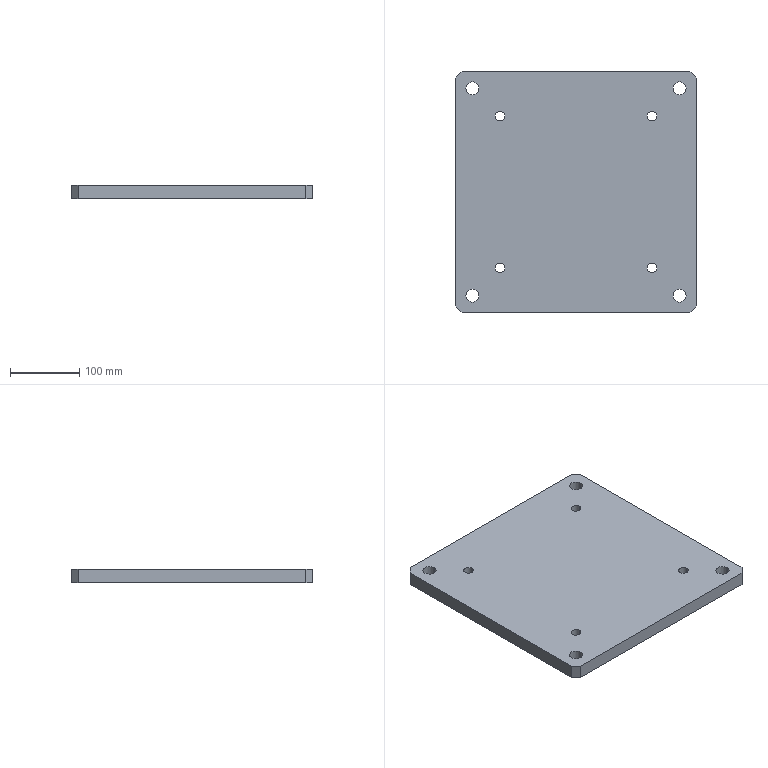Part | SolidWorks | features HoleWzd 2, Chamfer 1, Extrusion 1 | 1 solid | 26 faces | box 350 x 350 x 20 mm | volume 2411003 mm3 | cylinder 16 | plane 10 | commonest cylinder face diameters 14 x8 19 x8
STEP:
#1=CARTESIAN_POINT('',(140.5,150.,0.));
#2=VERTEX_POINT('',#1);
#3=CARTESIAN_POINT('',(159.5,150.,0.));
#4=VERTEX_POINT('',#3);
#5=CARTESIAN_POINT('',(150.,150.,0.));
#6=DIRECTION('',(0.,0.,1.));
#7=DIRECTION('',(1.,0.,0.));
#8=AXIS2_PLACEMENT_3D('',#5,#6,#7);
#9=CIRCLE('',#8,9.5);
#10=EDGE_CURVE('',#2,#4,#9,.T.);
#11=ORIENTED_EDGE('',*,*,#10,.F.);
#12=CARTESIAN_POINT('',(140.5,150.,20.));
#13=VERTEX_POINT('',#12);
#14=CARTESIAN_POINT('',(140.5,150.,20.));
#15=DIRECTION('',(0.,0.,1.));
#16=VECTOR('',#15,1000.);
#17=LINE('',#14,#16);
#18=EDGE_CURVE('',#2,#13,#17,.T.);
#19=ORIENTED_EDGE('',*,*,#18,.T.);
#20=CARTESIAN_POINT('',(159.5,150.,20.));
#21=VERTEX_POINT('',#20);
#22=CARTESIAN_POINT('',(150.,150.,20.));
#23=DIRECTION('',(0.,0.,1.));
#24=DIRECTION('',(1.,0.,0.));
#25=AXIS2_PLACEMENT_3D('',#22,#23,#24);
#26=CIRCLE('',#25,9.5);
#27=EDGE_CURVE('',#13,#21,#26,.T.);
#28=ORIENTED_EDGE('',*,*,#27,.T.);
#29=CARTESIAN_POINT('',(159.5,150.,20.));
#30=DIRECTION('',(0.,0.,1.));
#31=VECTOR('',#30,1000.);
#32=LINE('',#29,#31);
#33=EDGE_CURVE('',#4,#21,#32,.T.);
#34=ORIENTED_EDGE('',*,*,#33,.F.);
#35=EDGE_LOOP('',(#11,#19,#28,#34));
#36=FACE_OUTER_BOUND('',#35,.T.);
#37=CARTESIAN_POINT('',(150.,150.,20.));
#38=DIRECTION('',(0.,0.,1.));
#39=DIRECTION('',(1.,0.,0.));
#40=AXIS2_PLACEMENT_3D('',#37,#38,#39);
#41=CYLINDRICAL_SURFACE('',#40,9.5);
#42=ADVANCED_FACE('',(#36),#41,.F.);
#43=CARTESIAN_POINT('',(-159.5,-150.,0.));
#44=VERTEX_POINT('',#43);
#45=CARTESIAN_POINT('',(-140.5,-150.,0.));
#46=VERTEX_POINT('',#45);
#47=CARTESIAN_POINT('',(-150.,-150.,0.));
#48=DIRECTION('',(0.,0.,1.));
#49=DIRECTION('',(1.,0.,0.));
#50=AXIS2_PLACEMENT_3D('',#47,#48,#49);
#51=CIRCLE('',#50,9.5);
#52=EDGE_CURVE('',#44,#46,#51,.T.);
#53=ORIENTED_EDGE('',*,*,#52,.F.);
#54=CARTESIAN_POINT('',(-159.5,-150.,20.));
#55=VERTEX_POINT('',#54);
#56=CARTESIAN_POINT('',(-159.5,-150.,20.));
#57=DIRECTION('',(0.,0.,1.));
#58=VECTOR('',#57,1000.);
#59=LINE('',#56,#58);
#60=EDGE_CURVE('',#44,#55,#59,.T.);
#61=ORIENTED_EDGE('',*,*,#60,.T.);
#62=CARTESIAN_POINT('',(-140.5,-150.,20.));
#63=VERTEX_POINT('',#62);
#64=CARTESIAN_POINT('',(-150.,-150.,20.));
#65=DIRECTION('',(0.,0.,1.));
#66=DIRECTION('',(1.,0.,0.));
#67=AXIS2_PLACEMENT_3D('',#64,#65,#66);
#68=CIRCLE('',#67,9.5);
#69=EDGE_CURVE('',#55,#63,#68,.T.);
#70=ORIENTED_EDGE('',*,*,#69,.T.);
#71=CARTESIAN_POINT('',(-140.5,-150.,20.));
#72=DIRECTION('',(0.,0.,1.));
#73=VECTOR('',#72,1000.);
#74=LINE('',#71,#73);
#75=EDGE_CURVE('',#46,#63,#74,.T.);
#76=ORIENTED_EDGE('',*,*,#75,.F.);
#77=EDGE_LOOP('',(#53,#61,#70,#76));
#78=FACE_OUTER_BOUND('',#77,.T.);
#79=CARTESIAN_POINT('',(-150.,-150.,20.));
#80=DIRECTION('',(0.,0.,1.));
#81=DIRECTION('',(1.,0.,0.));
#82=AXIS2_PLACEMENT_3D('',#79,#80,#81);
#83=CYLINDRICAL_SURFACE('',#82,9.5);
#84=ADVANCED_FACE('',(#78),#83,.F.);
#85=CARTESIAN_POINT('',(-159.5,150.,0.));
#86=VERTEX_POINT('',#85);
#87=CARTESIAN_POINT('',(-140.5,150.,0.));
#88=VERTEX_POINT('',#87);
#89=CARTESIAN_POINT('',(-150.,150.,0.));
#90=DIRECTION('',(0.,0.,1.));
#91=DIRECTION('',(1.,0.,0.));
#92=AXIS2_PLACEMENT_3D('',#89,#90,#91);
#93=CIRCLE('',#92,9.5);
#94=EDGE_CURVE('',#86,#88,#93,.T.);
#95=ORIENTED_EDGE('',*,*,#94,.F.);
#96=CARTESIAN_POINT('',(-159.5,150.,20.));
#97=VERTEX_POINT('',#96);
#98=CARTESIAN_POINT('',(-159.5,150.,20.));
#99=DIRECTION('',(0.,0.,1.));
#100=VECTOR('',#99,1000.);
#101=LINE('',#98,#100);
#102=EDGE_CURVE('',#86,#97,#101,.T.);
#103=ORIENTED_EDGE('',*,*,#102,.T.);
#104=CARTESIAN_POINT('',(-140.5,150.,20.));
#105=VERTEX_POINT('',#104);
#106=CARTESIAN_POINT('',(-150.,150.,20.));
#107=DIRECTION('',(0.,0.,1.));
#108=DIRECTION('',(1.,0.,0.));
#109=AXIS2_PLACEMENT_3D('',#106,#107,#108);
#110=CIRCLE('',#109,9.5);
#111=EDGE_CURVE('',#97,#105,#110,.T.);
#112=ORIENTED_EDGE('',*,*,#111,.T.);
#113=CARTESIAN_POINT('',(-140.5,150.,20.));
#114=DIRECTION('',(0.,0.,1.));
#115=VECTOR('',#114,1000.);
#116=LINE('',#113,#115);
#117=EDGE_CURVE('',#88,#105,#116,.T.);
#118=ORIENTED_EDGE('',*,*,#117,.F.);
#119=EDGE_LOOP('',(#95,#103,#112,#118));
#120=FACE_OUTER_BOUND('',#119,.T.);
#121=CARTESIAN_POINT('',(-150.,150.,20.));
#122=DIRECTION('',(0.,0.,1.));
#123=DIRECTION('',(1.,0.,0.));
#124=AXIS2_PLACEMENT_3D('',#121,#122,#123);
#125=CYLINDRICAL_SURFACE('',#124,9.5);
#126=ADVANCED_FACE('',(#120),#125,.F.);
#127=CARTESIAN_POINT('',(140.5,-150.,0.));
#128=VERTEX_POINT('',#127);
#129=CARTESIAN_POINT('',(159.5,-150.,0.));
#130=VERTEX_POINT('',#129);
#131=CARTESIAN_POINT('',(150.,-150.,0.));
#132=DIRECTION('',(0.,0.,1.));
#133=DIRECTION('',(1.,0.,0.));
#134=AXIS2_PLACEMENT_3D('',#131,#132,#133);
#135=CIRCLE('',#134,9.5);
#136=EDGE_CURVE('',#128,#130,#135,.T.);
#137=ORIENTED_EDGE('',*,*,#136,.F.);
#138=CARTESIAN_POINT('',(140.5,-150.,20.));
#139=VERTEX_POINT('',#138);
#140=CARTESIAN_POINT('',(140.5,-150.,20.));
#141=DIRECTION('',(0.,0.,1.));
#142=VECTOR('',#141,1000.);
#143=LINE('',#140,#142);
#144=EDGE_CURVE('',#128,#139,#143,.T.);
#145=ORIENTED_EDGE('',*,*,#144,.T.);
#146=CARTESIAN_POINT('',(159.5,-150.,20.));
#147=VERTEX_POINT('',#146);
#148=CARTESIAN_POINT('',(150.,-150.,20.));
#149=DIRECTION('',(0.,0.,1.));
#150=DIRECTION('',(1.,0.,0.));
#151=AXIS2_PLACEMENT_3D('',#148,#149,#150);
#152=CIRCLE('',#151,9.5);
#153=EDGE_CURVE('',#139,#147,#152,.T.);
#154=ORIENTED_EDGE('',*,*,#153,.T.);
#155=CARTESIAN_POINT('',(159.5,-150.,20.));
#156=DIRECTION('',(0.,0.,1.));
#157=VECTOR('',#156,1000.);
#158=LINE('',#155,#157);
#159=EDGE_CURVE('',#130,#147,#158,.T.);
#160=ORIENTED_EDGE('',*,*,#159,.F.);
#161=EDGE_LOOP('',(#137,#145,#154,#160));
#162=FACE_OUTER_BOUND('',#161,.T.);
#163=CARTESIAN_POINT('',(150.,-150.,20.));
#164=DIRECTION('',(0.,0.,1.));
#165=DIRECTION('',(1.,0.,0.));
#166=AXIS2_PLACEMENT_3D('',#163,#164,#165);
#167=CYLINDRICAL_SURFACE('',#166,9.5);
#168=ADVANCED_FACE('',(#162),#167,.F.);
#169=CARTESIAN_POINT('',(103.,110.,0.));
#170=VERTEX_POINT('',#169);
#171=CARTESIAN_POINT('',(117.,110.,0.));
#172=VERTEX_POINT('',#171);
#173=CARTESIAN_POINT('',(110.,110.,0.));
#174=DIRECTION('',(0.,0.,1.));
#175=DIRECTION('',(1.,0.,0.));
#176=AXIS2_PLACEMENT_3D('',#173,#174,#175);
#177=CIRCLE('',#176,7.);
#178=EDGE_CURVE('',#170,#172,#177,.T.);
#179=ORIENTED_EDGE('',*,*,#178,.F.);
#180=CARTESIAN_POINT('',(103.,110.,20.));
#181=VERTEX_POINT('',#180);
#182=CARTESIAN_POINT('',(103.,110.,20.));
#183=DIRECTION('',(0.,0.,1.));
#184=VECTOR('',#183,1000.);
#185=LINE('',#182,#184);
#186=EDGE_CURVE('',#170,#181,#185,.T.);
#187=ORIENTED_EDGE('',*,*,#186,.T.);
#188=CARTESIAN_POINT('',(117.,110.,20.));
#189=VERTEX_POINT('',#188);
#190=CARTESIAN_POINT('',(110.,110.,20.));
#191=DIRECTION('',(0.,0.,1.));
#192=DIRECTION('',(1.,0.,0.));
#193=AXIS2_PLACEMENT_3D('',#190,#191,#192);
#194=CIRCLE('',#193,7.);
#195=EDGE_CURVE('',#181,#189,#194,.T.);
#196=ORIENTED_EDGE('',*,*,#195,.T.);
#197=CARTESIAN_POINT('',(117.,110.,20.));
#198=DIRECTION('',(0.,0.,1.));
#199=VECTOR('',#198,1000.);
#200=LINE('',#197,#199);
#201=EDGE_CURVE('',#172,#189,#200,.T.);
#202=ORIENTED_EDGE('',*,*,#201,.F.);
#203=EDGE_LOOP('',(#179,#187,#196,#202));
#204=FACE_OUTER_BOUND('',#203,.T.);
#205=CARTESIAN_POINT('',(110.,110.,20.));
#206=DIRECTION('',(0.,0.,1.));
#207=DIRECTION('',(1.,0.,0.));
#208=AXIS2_PLACEMENT_3D('',#205,#206,#207);
#209=CYLINDRICAL_SURFACE('',#208,7.);
#210=ADVANCED_FACE('',(#204),#209,.F.);
#211=CARTESIAN_POINT('',(-117.,-110.,0.));
#212=VERTEX_POINT('',#211);
#213=CARTESIAN_POINT('',(-103.,-110.,0.));
#214=VERTEX_POINT('',#213);
#215=CARTESIAN_POINT('',(-110.,-110.,0.));
#216=DIRECTION('',(0.,0.,1.));
#217=DIRECTION('',(1.,0.,0.));
#218=AXIS2_PLACEMENT_3D('',#215,#216,#217);
#219=CIRCLE('',#218,7.);
#220=EDGE_CURVE('',#212,#214,#219,.T.);
#221=ORIENTED_EDGE('',*,*,#220,.F.);
#222=CARTESIAN_POINT('',(-117.,-110.,20.));
#223=VERTEX_POINT('',#222);
#224=CARTESIAN_POINT('',(-117.,-110.,20.));
#225=DIRECTION('',(0.,0.,1.));
#226=VECTOR('',#225,1000.);
#227=LINE('',#224,#226);
#228=EDGE_CURVE('',#212,#223,#227,.T.);
#229=ORIENTED_EDGE('',*,*,#228,.T.);
#230=CARTESIAN_POINT('',(-103.,-110.,20.));
#231=VERTEX_POINT('',#230);
#232=CARTESIAN_POINT('',(-110.,-110.,20.));
#233=DIRECTION('',(0.,0.,1.));
#234=DIRECTION('',(1.,0.,0.));
#235=AXIS2_PLACEMENT_3D('',#232,#233,#234);
#236=CIRCLE('',#235,7.);
#237=EDGE_CURVE('',#223,#231,#236,.T.);
#238=ORIENTED_EDGE('',*,*,#237,.T.);
#239=CARTESIAN_POINT('',(-103.,-110.,20.));
#240=DIRECTION('',(0.,0.,1.));
#241=VECTOR('',#240,1000.);
#242=LINE('',#239,#241);
#243=EDGE_CURVE('',#214,#231,#242,.T.);
#244=ORIENTED_EDGE('',*,*,#243,.F.);
#245=EDGE_LOOP('',(#221,#229,#238,#244));
#246=FACE_OUTER_BOUND('',#245,.T.);
#247=CARTESIAN_POINT('',(-110.,-110.,20.));
#248=DIRECTION('',(0.,0.,1.));
#249=DIRECTION('',(1.,0.,0.));
#250=AXIS2_PLACEMENT_3D('',#247,#248,#249);
#251=CYLINDRICAL_SURFACE('',#250,7.);
#252=ADVANCED_FACE('',(#246),#251,.F.);
#253=CARTESIAN_POINT('',(-117.,110.,0.));
#254=VERTEX_POINT('',#253);
#255=CARTESIAN_POINT('',(-103.,110.,0.));
#256=VERTEX_POINT('',#255);
#257=CARTESIAN_POINT('',(-110.,110.,0.));
#258=DIRECTION('',(0.,0.,1.));
#259=DIRECTION('',(1.,0.,0.));
#260=AXIS2_PLACEMENT_3D('',#257,#258,#259);
#261=CIRCLE('',#260,7.);
#262=EDGE_CURVE('',#254,#256,#261,.T.);
#263=ORIENTED_EDGE('',*,*,#262,.F.);
#264=CARTESIAN_POINT('',(-117.,110.,20.));
#265=VERTEX_POINT('',#264);
#266=CARTESIAN_POINT('',(-117.,110.,20.));
#267=DIRECTION('',(0.,0.,1.));
#268=VECTOR('',#267,1000.);
#269=LINE('',#266,#268);
#270=EDGE_CURVE('',#254,#265,#269,.T.);
#271=ORIENTED_EDGE('',*,*,#270,.T.);
#272=CARTESIAN_POINT('',(-103.,110.,20.));
#273=VERTEX_POINT('',#272);
#274=CARTESIAN_POINT('',(-110.,110.,20.));
#275=DIRECTION('',(0.,0.,1.));
#276=DIRECTION('',(1.,0.,0.));
#277=AXIS2_PLACEMENT_3D('',#274,#275,#276);
#278=CIRCLE('',#277,7.);
#279=EDGE_CURVE('',#265,#273,#278,.T.);
#280=ORIENTED_EDGE('',*,*,#279,.T.);
#281=CARTESIAN_POINT('',(-103.,110.,20.));
#282=DIRECTION('',(0.,0.,1.));
#283=VECTOR('',#282,1000.);
#284=LINE('',#281,#283);
#285=EDGE_CURVE('',#256,#273,#284,.T.);
#286=ORIENTED_EDGE('',*,*,#285,.F.);
#287=EDGE_LOOP('',(#263,#271,#280,#286));
#288=FACE_OUTER_BOUND('',#287,.T.);
#289=CARTESIAN_POINT('',(-110.,110.,20.));
#290=DIRECTION('',(0.,0.,1.));
#291=DIRECTION('',(1.,0.,0.));
#292=AXIS2_PLACEMENT_3D('',#289,#290,#291);
#293=CYLINDRICAL_SURFACE('',#292,7.);
#294=ADVANCED_FACE('',(#288),#293,.F.);
#295=CARTESIAN_POINT('',(103.,-110.,0.));
#296=VERTEX_POINT('',#295);
#297=CARTESIAN_POINT('',(117.,-110.,0.));
#298=VERTEX_POINT('',#297);
#299=CARTESIAN_POINT('',(110.,-110.,0.));
#300=DIRECTION('',(0.,0.,1.));
#301=DIRECTION('',(1.,0.,0.));
#302=AXIS2_PLACEMENT_3D('',#299,#300,#301);
#303=CIRCLE('',#302,7.);
#304=EDGE_CURVE('',#296,#298,#303,.T.);
#305=ORIENTED_EDGE('',*,*,#304,.F.);
#306=CARTESIAN_POINT('',(103.,-110.,20.));
#307=VERTEX_POINT('',#306);
#308=CARTESIAN_POINT('',(103.,-110.,20.));
#309=DIRECTION('',(0.,0.,1.));
#310=VECTOR('',#309,1000.);
#311=LINE('',#308,#310);
#312=EDGE_CURVE('',#296,#307,#311,.T.);
#313=ORIENTED_EDGE('',*,*,#312,.T.);
#314=CARTESIAN_POINT('',(117.,-110.,20.));
#315=VERTEX_POINT('',#314);
#316=CARTESIAN_POINT('',(110.,-110.,20.));
#317=DIRECTION('',(0.,0.,1.));
#318=DIRECTION('',(1.,0.,0.));
#319=AXIS2_PLACEMENT_3D('',#316,#317,#318);
#320=CIRCLE('',#319,7.);
#321=EDGE_CURVE('',#307,#315,#320,.T.);
#322=ORIENTED_EDGE('',*,*,#321,.T.);
#323=CARTESIAN_POINT('',(117.,-110.,20.));
#324=DIRECTION('',(0.,0.,1.));
#325=VECTOR('',#324,1000.);
#326=LINE('',#323,#325);
#327=EDGE_CURVE('',#298,#315,#326,.T.);
#328=ORIENTED_EDGE('',*,*,#327,.F.);
#329=EDGE_LOOP('',(#305,#313,#322,#328));
#330=FACE_OUTER_BOUND('',#329,.T.);
#331=CARTESIAN_POINT('',(110.,-110.,20.));
#332=DIRECTION('',(0.,0.,1.));
#333=DIRECTION('',(1.,0.,0.));
#334=AXIS2_PLACEMENT_3D('',#331,#332,#333);
#335=CYLINDRICAL_SURFACE('',#334,7.);
#336=ADVANCED_FACE('',(#330),#335,.F.);
#337=CARTESIAN_POINT('',(175.,-165.,20.));
#338=VERTEX_POINT('',#337);
#339=CARTESIAN_POINT('',(175.,165.,20.));
#340=VERTEX_POINT('',#339);
#341=CARTESIAN_POINT('',(175.,175.,20.));
#342=DIRECTION('',(0.,1.,0.));
#343=VECTOR('',#342,1000.);
#344=LINE('',#341,#343);
#345=EDGE_CURVE('',#338,#340,#344,.T.);
#346=ORIENTED_EDGE('',*,*,#345,.F.);
#347=CARTESIAN_POINT('',(175.,-165.,0.));
#348=VERTEX_POINT('',#347);
#349=CARTESIAN_POINT('',(175.,-165.,20.));
#350=DIRECTION('',(0.,0.,-1.));
#351=VECTOR('',#350,1000.);
#352=LINE('',#349,#351);
#353=EDGE_CURVE('',#338,#348,#352,.T.);
#354=ORIENTED_EDGE('',*,*,#353,.T.);
#355=CARTESIAN_POINT('',(175.,165.,0.));
#356=VERTEX_POINT('',#355);
#357=CARTESIAN_POINT('',(175.,175.,0.));
#358=DIRECTION('',(0.,1.,0.));
#359=VECTOR('',#358,1000.);
#360=LINE('',#357,#359);
#361=EDGE_CURVE('',#348,#356,#360,.T.);
#362=ORIENTED_EDGE('',*,*,#361,.T.);
#363=CARTESIAN_POINT('',(175.,165.,20.));
#364=DIRECTION('',(0.,0.,1.));
#365=VECTOR('',#364,1000.);
#366=LINE('',#363,#365);
#367=EDGE_CURVE('',#356,#340,#366,.T.);
#368=ORIENTED_EDGE('',*,*,#367,.T.);
#369=EDGE_LOOP('',(#346,#354,#362,#368));
#370=FACE_OUTER_BOUND('',#369,.T.);
#371=CARTESIAN_POINT('',(175.,175.,20.));
#372=DIRECTION('',(-1.,0.,0.));
#373=DIRECTION('',(0.,0.,1.));
#374=AXIS2_PLACEMENT_3D('',#371,#372,#373);
#375=PLANE('',#374);
#376=ADVANCED_FACE('',(#370),#375,.F.);
#377=CARTESIAN_POINT('',(165.,175.,20.));
#378=VERTEX_POINT('',#377);
#379=CARTESIAN_POINT('',(-165.,175.,20.));
#380=VERTEX_POINT('',#379);
#381=CARTESIAN_POINT('',(-175.,175.,20.));
#382=DIRECTION('',(-1.,0.,0.));
#383=VECTOR('',#382,1000.);
#384=LINE('',#381,#383);
#385=EDGE_CURVE('',#378,#380,#384,.T.);
#386=ORIENTED_EDGE('',*,*,#385,.F.);
#387=CARTESIAN_POINT('',(165.,175.,0.));
#388=VERTEX_POINT('',#387);
#389=CARTESIAN_POINT('',(165.,175.,20.));
#390=DIRECTION('',(0.,0.,-1.));
#391=VECTOR('',#390,1000.);
#392=LINE('',#389,#391);
#393=EDGE_CURVE('',#378,#388,#392,.T.);
#394=ORIENTED_EDGE('',*,*,#393,.T.);
#395=CARTESIAN_POINT('',(-165.,175.,0.));
#396=VERTEX_POINT('',#395);
#397=CARTESIAN_POINT('',(-175.,175.,0.));
#398=DIRECTION('',(-1.,0.,0.));
#399=VECTOR('',#398,1000.);
#400=LINE('',#397,#399);
#401=EDGE_CURVE('',#388,#396,#400,.T.);
#402=ORIENTED_EDGE('',*,*,#401,.T.);
#403=CARTESIAN_POINT('',(-165.,175.,20.));
#404=DIRECTION('',(0.,0.,1.));
#405=VECTOR('',#404,1000.);
#406=LINE('',#403,#405);
#407=EDGE_CURVE('',#396,#380,#406,.T.);
#408=ORIENTED_EDGE('',*,*,#407,.T.);
#409=EDGE_LOOP('',(#386,#394,#402,#408));
#410=FACE_OUTER_BOUND('',#409,.T.);
#411=CARTESIAN_POINT('',(-175.,175.,20.));
#412=DIRECTION('',(0.,-1.,0.));
#413=DIRECTION('',(0.,0.,-1.));
#414=AXIS2_PLACEMENT_3D('',#411,#412,#413);
#415=PLANE('',#414);
#416=ADVANCED_FACE('',(#410),#415,.F.);
#417=CARTESIAN_POINT('',(-175.,165.,0.));
#418=VERTEX_POINT('',#417);
#419=CARTESIAN_POINT('',(-175.,-165.,0.));
#420=VERTEX_POINT('',#419);
#421=CARTESIAN_POINT('',(-175.,175.,0.));
#422=DIRECTION('',(0.,-1.,0.));
#423=VECTOR('',#422,1000.);
#424=LINE('',#421,#423);
#425=EDGE_CURVE('',#418,#420,#424,.T.);
#426=ORIENTED_EDGE('',*,*,#425,.T.);
#427=CARTESIAN_POINT('',(-175.,-165.,20.));
#428=VERTEX_POINT('',#427);
#429=CARTESIAN_POINT('',(-175.,-165.,20.));
#430=DIRECTION('',(0.,0.,1.));
#431=VECTOR('',#430,1000.);
#432=LINE('',#429,#431);
#433=EDGE_CURVE('',#420,#428,#432,.T.);
#434=ORIENTED_EDGE('',*,*,#433,.T.);
#435=CARTESIAN_POINT('',(-175.,165.,20.));
#436=VERTEX_POINT('',#435);
#437=CARTESIAN_POINT('',(-175.,175.,20.));
#438=DIRECTION('',(0.,-1.,0.));
#439=VECTOR('',#438,1000.);
#440=LINE('',#437,#439);
#441=EDGE_CURVE('',#436,#428,#440,.T.);
#442=ORIENTED_EDGE('',*,*,#441,.F.);
#443=CARTESIAN_POINT('',(-175.,165.,20.));
#444=DIRECTION('',(0.,0.,-1.));
#445=VECTOR('',#444,1000.);
#446=LINE('',#443,#445);
#447=EDGE_CURVE('',#436,#418,#446,.T.);
#448=ORIENTED_EDGE('',*,*,#447,.T.);
#449=EDGE_LOOP('',(#426,#434,#442,#448));
#450=FACE_OUTER_BOUND('',#449,.T.);
#451=CARTESIAN_POINT('',(-175.,175.,20.));
#452=DIRECTION('',(1.,0.,0.));
#453=DIRECTION('',(0.,0.,-1.));
#454=AXIS2_PLACEMENT_3D('',#451,#452,#453);
#455=PLANE('',#454);
#456=ADVANCED_FACE('',(#450),#455,.F.);
#457=CARTESIAN_POINT('',(-165.,-175.,20.));
#458=VERTEX_POINT('',#457);
#459=CARTESIAN_POINT('',(165.,-175.,20.));
#460=VERTEX_POINT('',#459);
#461=CARTESIAN_POINT('',(-175.,-175.,20.));
#462=DIRECTION('',(1.,0.,0.));
#463=VECTOR('',#462,1000.);
#464=LINE('',#461,#463);
#465=EDGE_CURVE('',#458,#460,#464,.T.);
#466=ORIENTED_EDGE('',*,*,#465,.F.);
#467=CARTESIAN_POINT('',(-165.,-175.,0.));
#468=VERTEX_POINT('',#467);
#469=CARTESIAN_POINT('',(-165.,-175.,20.));
#470=DIRECTION('',(0.,0.,-1.));
#471=VECTOR('',#470,1000.);
#472=LINE('',#469,#471);
#473=EDGE_CURVE('',#458,#468,#472,.T.);
#474=ORIENTED_EDGE('',*,*,#473,.T.);
#475=CARTESIAN_POINT('',(165.,-175.,0.));
#476=VERTEX_POINT('',#475);
#477=CARTESIAN_POINT('',(-175.,-175.,0.));
#478=DIRECTION('',(1.,0.,0.));
#479=VECTOR('',#478,1000.);
#480=LINE('',#477,#479);
#481=EDGE_CURVE('',#468,#476,#480,.T.);
#482=ORIENTED_EDGE('',*,*,#481,.T.);
#483=CARTESIAN_POINT('',(165.,-175.,20.));
#484=DIRECTION('',(0.,0.,1.));
#485=VECTOR('',#484,1000.);
#486=LINE('',#483,#485);
#487=EDGE_CURVE('',#476,#460,#486,.T.);
#488=ORIENTED_EDGE('',*,*,#487,.T.);
#489=EDGE_LOOP('',(#466,#474,#482,#488));
#490=FACE_OUTER_BOUND('',#489,.T.);
#491=CARTESIAN_POINT('',(-175.,-175.,20.));
#492=DIRECTION('',(0.,1.,0.));
#493=DIRECTION('',(0.,0.,1.));
#494=AXIS2_PLACEMENT_3D('',#491,#492,#493);
#495=PLANE('',#494);
#496=ADVANCED_FACE('',(#490),#495,.F.);
#497=CARTESIAN_POINT('',(150.,150.,20.));
#498=DIRECTION('',(0.,0.,1.));
#499=DIRECTION('',(1.,0.,0.));
#500=AXIS2_PLACEMENT_3D('',#497,#498,#499);
#501=CIRCLE('',#500,9.5);
#502=EDGE_CURVE('',#21,#13,#501,.T.);
#503=ORIENTED_EDGE('',*,*,#502,.F.);
#504=ORIENTED_EDGE('',*,*,#27,.F.);
#505=EDGE_LOOP('',(#503,#504));
#506=FACE_BOUND('',#505,.T.);
#507=CARTESIAN_POINT('',(-150.,-150.,20.));
#508=DIRECTION('',(0.,0.,1.));
#509=DIRECTION('',(1.,0.,0.));
#510=AXIS2_PLACEMENT_3D('',#507,#508,#509);
#511=CIRCLE('',#510,9.5);
#512=EDGE_CURVE('',#63,#55,#511,.T.);
#513=ORIENTED_EDGE('',*,*,#512,.F.);
#514=ORIENTED_EDGE('',*,*,#69,.F.);
#515=EDGE_LOOP('',(#513,#514));
#516=FACE_BOUND('',#515,.T.);
#517=CARTESIAN_POINT('',(-150.,150.,20.));
#518=DIRECTION('',(0.,0.,1.));
#519=DIRECTION('',(1.,0.,0.));
#520=AXIS2_PLACEMENT_3D('',#517,#518,#519);
#521=CIRCLE('',#520,9.5);
#522=EDGE_CURVE('',#105,#97,#521,.T.);
#523=ORIENTED_EDGE('',*,*,#522,.F.);
#524=ORIENTED_EDGE('',*,*,#111,.F.);
#525=EDGE_LOOP('',(#523,#524));
#526=FACE_BOUND('',#525,.T.);
#527=CARTESIAN_POINT('',(150.,-150.,20.));
#528=DIRECTION('',(0.,0.,1.));
#529=DIRECTION('',(1.,0.,0.));
#530=AXIS2_PLACEMENT_3D('',#527,#528,#529);
#531=CIRCLE('',#530,9.5);
#532=EDGE_CURVE('',#147,#139,#531,.T.);
#533=ORIENTED_EDGE('',*,*,#532,.F.);
#534=ORIENTED_EDGE('',*,*,#153,.F.);
#535=EDGE_LOOP('',(#533,#534));
#536=FACE_BOUND('',#535,.T.);
#537=CARTESIAN_POINT('',(110.,110.,20.));
#538=DIRECTION('',(0.,0.,1.));
#539=DIRECTION('',(1.,0.,0.));
#540=AXIS2_PLACEMENT_3D('',#537,#538,#539);
#541=CIRCLE('',#540,7.);
#542=EDGE_CURVE('',#189,#181,#541,.T.);
#543=ORIENTED_EDGE('',*,*,#542,.F.);
#544=ORIENTED_EDGE('',*,*,#195,.F.);
#545=EDGE_LOOP('',(#543,#544));
#546=FACE_BOUND('',#545,.T.);
#547=CARTESIAN_POINT('',(-110.,-110.,20.));
#548=DIRECTION('',(0.,0.,1.));
#549=DIRECTION('',(1.,0.,0.));
#550=AXIS2_PLACEMENT_3D('',#547,#548,#549);
#551=CIRCLE('',#550,7.);
#552=EDGE_CURVE('',#231,#223,#551,.T.);
#553=ORIENTED_EDGE('',*,*,#552,.F.);
#554=ORIENTED_EDGE('',*,*,#237,.F.);
#555=EDGE_LOOP('',(#553,#554));
#556=FACE_BOUND('',#555,.T.);
#557=CARTESIAN_POINT('',(-110.,110.,20.));
#558=DIRECTION('',(0.,0.,1.));
#559=DIRECTION('',(1.,0.,0.));
#560=AXIS2_PLACEMENT_3D('',#557,#558,#559);
#561=CIRCLE('',#560,7.);
#562=EDGE_CURVE('',#273,#265,#561,.T.);
#563=ORIENTED_EDGE('',*,*,#562,.F.);
#564=ORIENTED_EDGE('',*,*,#279,.F.);
#565=EDGE_LOOP('',(#563,#564));
#566=FACE_BOUND('',#565,.T.);
#567=CARTESIAN_POINT('',(110.,-110.,20.));
#568=DIRECTION('',(0.,0.,1.));
#569=DIRECTION('',(1.,0.,0.));
#570=AXIS2_PLACEMENT_3D('',#567,#568,#569);
#571=CIRCLE('',#570,7.);
#572=EDGE_CURVE('',#315,#307,#571,.T.);
#573=ORIENTED_EDGE('',*,*,#572,.F.);
#574=ORIENTED_EDGE('',*,*,#321,.F.);
#575=EDGE_LOOP('',(#573,#574));
#576=FACE_BOUND('',#575,.T.);
#577=ORIENTED_EDGE('',*,*,#441,.T.);
#578=CARTESIAN_POINT('',(-170.,-170.,20.));
#579=DIRECTION('',(0.7071,-0.7071,0.));
#580=VECTOR('',#579,1000.);
#581=LINE('',#578,#580);
#582=EDGE_CURVE('',#428,#458,#581,.T.);
#583=ORIENTED_EDGE('',*,*,#582,.T.);
#584=ORIENTED_EDGE('',*,*,#465,.T.);
#585=CARTESIAN_POINT('',(170.,-170.,20.));
#586=DIRECTION('',(0.7071,0.7071,0.));
#587=VECTOR('',#586,1000.);
#588=LINE('',#585,#587);
#589=EDGE_CURVE('',#460,#338,#588,.T.);
#590=ORIENTED_EDGE('',*,*,#589,.T.);
#591=ORIENTED_EDGE('',*,*,#345,.T.);
#592=CARTESIAN_POINT('',(170.,170.,20.));
#593=DIRECTION('',(-0.7071,0.7071,0.));
#594=VECTOR('',#593,1000.);
#595=LINE('',#592,#594);
#596=EDGE_CURVE('',#340,#378,#595,.T.);
#597=ORIENTED_EDGE('',*,*,#596,.T.);
#598=ORIENTED_EDGE('',*,*,#385,.T.);
#599=CARTESIAN_POINT('',(-170.,170.,20.));
#600=DIRECTION('',(-0.7071,-0.7071,0.));
#601=VECTOR('',#600,1000.);
#602=LINE('',#599,#601);
#603=EDGE_CURVE('',#380,#436,#602,.T.);
#604=ORIENTED_EDGE('',*,*,#603,.T.);
#605=EDGE_LOOP('',(#577,#583,#584,#590,#591,#597,#598,#604));
#606=FACE_OUTER_BOUND('',#605,.T.);
#607=CARTESIAN_POINT('',(0.,0.,20.));
#608=DIRECTION('',(0.,0.,1.));
#609=DIRECTION('',(1.,0.,0.));
#610=AXIS2_PLACEMENT_3D('',#607,#608,#609);
#611=PLANE('',#610);
#612=ADVANCED_FACE('',(#506,#516,#526,#536,#546,#556,#566,#576,#606),#611,.T.);
#613=CARTESIAN_POINT('',(150.,150.,0.));
#614=DIRECTION('',(0.,0.,1.));
#615=DIRECTION('',(1.,0.,0.));
#616=AXIS2_PLACEMENT_3D('',#613,#614,#615);
#617=CIRCLE('',#616,9.5);
#618=EDGE_CURVE('',#4,#2,#617,.T.);
#619=ORIENTED_EDGE('',*,*,#618,.T.);
#620=ORIENTED_EDGE('',*,*,#10,.T.);
#621=EDGE_LOOP('',(#619,#620));
#622=FACE_BOUND('',#621,.T.);
#623=CARTESIAN_POINT('',(-150.,-150.,0.));
#624=DIRECTION('',(0.,0.,1.));
#625=DIRECTION('',(1.,0.,0.));
#626=AXIS2_PLACEMENT_3D('',#623,#624,#625);
#627=CIRCLE('',#626,9.5);
#628=EDGE_CURVE('',#46,#44,#627,.T.);
#629=ORIENTED_EDGE('',*,*,#628,.T.);
#630=ORIENTED_EDGE('',*,*,#52,.T.);
#631=EDGE_LOOP('',(#629,#630));
#632=FACE_BOUND('',#631,.T.);
#633=CARTESIAN_POINT('',(-150.,150.,0.));
#634=DIRECTION('',(0.,0.,1.));
#635=DIRECTION('',(1.,0.,0.));
#636=AXIS2_PLACEMENT_3D('',#633,#634,#635);
#637=CIRCLE('',#636,9.5);
#638=EDGE_CURVE('',#88,#86,#637,.T.);
#639=ORIENTED_EDGE('',*,*,#638,.T.);
#640=ORIENTED_EDGE('',*,*,#94,.T.);
#641=EDGE_LOOP('',(#639,#640));
#642=FACE_BOUND('',#641,.T.);
#643=CARTESIAN_POINT('',(150.,-150.,0.));
#644=DIRECTION('',(0.,0.,1.));
#645=DIRECTION('',(1.,0.,0.));
#646=AXIS2_PLACEMENT_3D('',#643,#644,#645);
#647=CIRCLE('',#646,9.5);
#648=EDGE_CURVE('',#130,#128,#647,.T.);
#649=ORIENTED_EDGE('',*,*,#648,.T.);
#650=ORIENTED_EDGE('',*,*,#136,.T.);
#651=EDGE_LOOP('',(#649,#650));
#652=FACE_BOUND('',#651,.T.);
#653=CARTESIAN_POINT('',(110.,110.,0.));
#654=DIRECTION('',(0.,0.,1.));
#655=DIRECTION('',(1.,0.,0.));
#656=AXIS2_PLACEMENT_3D('',#653,#654,#655);
#657=CIRCLE('',#656,7.);
#658=EDGE_CURVE('',#172,#170,#657,.T.);
#659=ORIENTED_EDGE('',*,*,#658,.T.);
#660=ORIENTED_EDGE('',*,*,#178,.T.);
#661=EDGE_LOOP('',(#659,#660));
#662=FACE_BOUND('',#661,.T.);
#663=CARTESIAN_POINT('',(-110.,-110.,0.));
#664=DIRECTION('',(0.,0.,1.));
#665=DIRECTION('',(1.,0.,0.));
#666=AXIS2_PLACEMENT_3D('',#663,#664,#665);
#667=CIRCLE('',#666,7.);
#668=EDGE_CURVE('',#214,#212,#667,.T.);
#669=ORIENTED_EDGE('',*,*,#668,.T.);
#670=ORIENTED_EDGE('',*,*,#220,.T.);
#671=EDGE_LOOP('',(#669,#670));
#672=FACE_BOUND('',#671,.T.);
#673=CARTESIAN_POINT('',(-110.,110.,0.));
#674=DIRECTION('',(0.,0.,1.));
#675=DIRECTION('',(1.,0.,0.));
#676=AXIS2_PLACEMENT_3D('',#673,#674,#675);
#677=CIRCLE('',#676,7.);
#678=EDGE_CURVE('',#256,#254,#677,.T.);
#679=ORIENTED_EDGE('',*,*,#678,.T.);
#680=ORIENTED_EDGE('',*,*,#262,.T.);
#681=EDGE_LOOP('',(#679,#680));
#682=FACE_BOUND('',#681,.T.);
#683=CARTESIAN_POINT('',(110.,-110.,0.));
#684=DIRECTION('',(0.,0.,1.));
#685=DIRECTION('',(1.,0.,0.));
#686=AXIS2_PLACEMENT_3D('',#683,#684,#685);
#687=CIRCLE('',#686,7.);
#688=EDGE_CURVE('',#298,#296,#687,.T.);
#689=ORIENTED_EDGE('',*,*,#688,.T.);
#690=ORIENTED_EDGE('',*,*,#304,.T.);
#691=EDGE_LOOP('',(#689,#690));
#692=FACE_BOUND('',#691,.T.);
#693=ORIENTED_EDGE('',*,*,#481,.F.);
#694=CARTESIAN_POINT('',(-165.,-175.,0.));
#695=DIRECTION('',(-0.7071,0.7071,0.));
#696=VECTOR('',#695,1000.);
#697=LINE('',#694,#696);
#698=EDGE_CURVE('',#468,#420,#697,.T.);
#699=ORIENTED_EDGE('',*,*,#698,.T.);
#700=ORIENTED_EDGE('',*,*,#425,.F.);
#701=CARTESIAN_POINT('',(-175.,165.,0.));
#702=DIRECTION('',(0.7071,0.7071,0.));
#703=VECTOR('',#702,1000.);
#704=LINE('',#701,#703);
#705=EDGE_CURVE('',#418,#396,#704,.T.);
#706=ORIENTED_EDGE('',*,*,#705,.T.);
#707=ORIENTED_EDGE('',*,*,#401,.F.);
#708=CARTESIAN_POINT('',(165.,175.,0.));
#709=DIRECTION('',(0.7071,-0.7071,0.));
#710=VECTOR('',#709,1000.);
#711=LINE('',#708,#710);
#712=EDGE_CURVE('',#388,#356,#711,.T.);
#713=ORIENTED_EDGE('',*,*,#712,.T.);
#714=ORIENTED_EDGE('',*,*,#361,.F.);
#715=CARTESIAN_POINT('',(175.,-165.,0.));
#716=DIRECTION('',(-0.7071,-0.7071,0.));
#717=VECTOR('',#716,1000.);
#718=LINE('',#715,#717);
#719=EDGE_CURVE('',#348,#476,#718,.T.);
#720=ORIENTED_EDGE('',*,*,#719,.T.);
#721=EDGE_LOOP('',(#693,#699,#700,#706,#707,#713,#714,#720));
#722=FACE_OUTER_BOUND('',#721,.T.);
#723=CARTESIAN_POINT('',(0.,0.,0.));
#724=DIRECTION('',(0.,0.,1.));
#725=DIRECTION('',(1.,0.,0.));
#726=AXIS2_PLACEMENT_3D('',#723,#724,#725);
#727=PLANE('',#726);
#728=ADVANCED_FACE('',(#622,#632,#642,#652,#662,#672,#682,#692,#722),#727,.F.);
#729=ORIENTED_EDGE('',*,*,#312,.F.);
#730=ORIENTED_EDGE('',*,*,#688,.F.);
#731=ORIENTED_EDGE('',*,*,#327,.T.);
#732=ORIENTED_EDGE('',*,*,#572,.T.);
#733=EDGE_LOOP('',(#729,#730,#731,#732));
#734=FACE_OUTER_BOUND('',#733,.T.);
#735=CARTESIAN_POINT('',(110.,-110.,20.));
#736=DIRECTION('',(0.,0.,1.));
#737=DIRECTION('',(1.,0.,0.));
#738=AXIS2_PLACEMENT_3D('',#735,#736,#737);
#739=CYLINDRICAL_SURFACE('',#738,7.);
#740=ADVANCED_FACE('',(#734),#739,.F.);
#741=ORIENTED_EDGE('',*,*,#270,.F.);
#742=ORIENTED_EDGE('',*,*,#678,.F.);
#743=ORIENTED_EDGE('',*,*,#285,.T.);
#744=ORIENTED_EDGE('',*,*,#562,.T.);
#745=EDGE_LOOP('',(#741,#742,#743,#744));
#746=FACE_OUTER_BOUND('',#745,.T.);
#747=CARTESIAN_POINT('',(-110.,110.,20.));
#748=DIRECTION('',(0.,0.,1.));
#749=DIRECTION('',(1.,0.,0.));
#750=AXIS2_PLACEMENT_3D('',#747,#748,#749);
#751=CYLINDRICAL_SURFACE('',#750,7.);
#752=ADVANCED_FACE('',(#746),#751,.F.);
#753=ORIENTED_EDGE('',*,*,#228,.F.);
#754=ORIENTED_EDGE('',*,*,#668,.F.);
#755=ORIENTED_EDGE('',*,*,#243,.T.);
#756=ORIENTED_EDGE('',*,*,#552,.T.);
#757=EDGE_LOOP('',(#753,#754,#755,#756));
#758=FACE_OUTER_BOUND('',#757,.T.);
#759=CARTESIAN_POINT('',(-110.,-110.,20.));
#760=DIRECTION('',(0.,0.,1.));
#761=DIRECTION('',(1.,0.,0.));
#762=AXIS2_PLACEMENT_3D('',#759,#760,#761);
#763=CYLINDRICAL_SURFACE('',#762,7.);
#764=ADVANCED_FACE('',(#758),#763,.F.);
#765=ORIENTED_EDGE('',*,*,#186,.F.);
#766=ORIENTED_EDGE('',*,*,#658,.F.);
#767=ORIENTED_EDGE('',*,*,#201,.T.);
#768=ORIENTED_EDGE('',*,*,#542,.T.);
#769=EDGE_LOOP('',(#765,#766,#767,#768));
#770=FACE_OUTER_BOUND('',#769,.T.);
#771=CARTESIAN_POINT('',(110.,110.,20.));
#772=DIRECTION('',(0.,0.,1.));
#773=DIRECTION('',(1.,0.,0.));
#774=AXIS2_PLACEMENT_3D('',#771,#772,#773);
#775=CYLINDRICAL_SURFACE('',#774,7.);
#776=ADVANCED_FACE('',(#770),#775,.F.);
#777=ORIENTED_EDGE('',*,*,#144,.F.);
#778=ORIENTED_EDGE('',*,*,#648,.F.);
#779=ORIENTED_EDGE('',*,*,#159,.T.);
#780=ORIENTED_EDGE('',*,*,#532,.T.);
#781=EDGE_LOOP('',(#777,#778,#779,#780));
#782=FACE_OUTER_BOUND('',#781,.T.);
#783=CARTESIAN_POINT('',(150.,-150.,20.));
#784=DIRECTION('',(0.,0.,1.));
#785=DIRECTION('',(1.,0.,0.));
#786=AXIS2_PLACEMENT_3D('',#783,#784,#785);
#787=CYLINDRICAL_SURFACE('',#786,9.5);
#788=ADVANCED_FACE('',(#782),#787,.F.);
#789=ORIENTED_EDGE('',*,*,#102,.F.);
#790=ORIENTED_EDGE('',*,*,#638,.F.);
#791=ORIENTED_EDGE('',*,*,#117,.T.);
#792=ORIENTED_EDGE('',*,*,#522,.T.);
#793=EDGE_LOOP('',(#789,#790,#791,#792));
#794=FACE_OUTER_BOUND('',#793,.T.);
#795=CARTESIAN_POINT('',(-150.,150.,20.));
#796=DIRECTION('',(0.,0.,1.));
#797=DIRECTION('',(1.,0.,0.));
#798=AXIS2_PLACEMENT_3D('',#795,#796,#797);
#799=CYLINDRICAL_SURFACE('',#798,9.5);
#800=ADVANCED_FACE('',(#794),#799,.F.);
#801=ORIENTED_EDGE('',*,*,#60,.F.);
#802=ORIENTED_EDGE('',*,*,#628,.F.);
#803=ORIENTED_EDGE('',*,*,#75,.T.);
#804=ORIENTED_EDGE('',*,*,#512,.T.);
#805=EDGE_LOOP('',(#801,#802,#803,#804));
#806=FACE_OUTER_BOUND('',#805,.T.);
#807=CARTESIAN_POINT('',(-150.,-150.,20.));
#808=DIRECTION('',(0.,0.,1.));
#809=DIRECTION('',(1.,0.,0.));
#810=AXIS2_PLACEMENT_3D('',#807,#808,#809);
#811=CYLINDRICAL_SURFACE('',#810,9.5);
#812=ADVANCED_FACE('',(#806),#811,.F.);
#813=ORIENTED_EDGE('',*,*,#18,.F.);
#814=ORIENTED_EDGE('',*,*,#618,.F.);
#815=ORIENTED_EDGE('',*,*,#33,.T.);
#816=ORIENTED_EDGE('',*,*,#502,.T.);
#817=EDGE_LOOP('',(#813,#814,#815,#816));
#818=FACE_OUTER_BOUND('',#817,.T.);
#819=CARTESIAN_POINT('',(150.,150.,20.));
#820=DIRECTION('',(0.,0.,1.));
#821=DIRECTION('',(1.,0.,0.));
#822=AXIS2_PLACEMENT_3D('',#819,#820,#821);
#823=CYLINDRICAL_SURFACE('',#822,9.5);
#824=ADVANCED_FACE('',(#818),#823,.F.);
#825=ORIENTED_EDGE('',*,*,#582,.F.);
#826=ORIENTED_EDGE('',*,*,#433,.F.);
#827=ORIENTED_EDGE('',*,*,#698,.F.);
#828=ORIENTED_EDGE('',*,*,#473,.F.);
#829=EDGE_LOOP('',(#825,#826,#827,#828));
#830=FACE_OUTER_BOUND('',#829,.T.);
#831=CARTESIAN_POINT('',(-165.,-175.,20.));
#832=DIRECTION('',(0.7071,0.7071,0.));
#833=DIRECTION('',(0.,0.,-1.));
#834=AXIS2_PLACEMENT_3D('',#831,#832,#833);
#835=PLANE('',#834);
#836=ADVANCED_FACE('',(#830),#835,.F.);
#837=ORIENTED_EDGE('',*,*,#589,.F.);
#838=ORIENTED_EDGE('',*,*,#487,.F.);
#839=ORIENTED_EDGE('',*,*,#719,.F.);
#840=ORIENTED_EDGE('',*,*,#353,.F.);
#841=EDGE_LOOP('',(#837,#838,#839,#840));
#842=FACE_OUTER_BOUND('',#841,.T.);
#843=CARTESIAN_POINT('',(175.,-165.,20.));
#844=DIRECTION('',(-0.7071,0.7071,0.));
#845=DIRECTION('',(0.,0.,-1.));
#846=AXIS2_PLACEMENT_3D('',#843,#844,#845);
#847=PLANE('',#846);
#848=ADVANCED_FACE('',(#842),#847,.F.);
#849=ORIENTED_EDGE('',*,*,#596,.F.);
#850=ORIENTED_EDGE('',*,*,#367,.F.);
#851=ORIENTED_EDGE('',*,*,#712,.F.);
#852=ORIENTED_EDGE('',*,*,#393,.F.);
#853=EDGE_LOOP('',(#849,#850,#851,#852));
#854=FACE_OUTER_BOUND('',#853,.T.);
#855=CARTESIAN_POINT('',(165.,175.,20.));
#856=DIRECTION('',(-0.7071,-0.7071,0.));
#857=DIRECTION('',(0.,0.,-1.));
#858=AXIS2_PLACEMENT_3D('',#855,#856,#857);
#859=PLANE('',#858);
#860=ADVANCED_FACE('',(#854),#859,.F.);
#861=ORIENTED_EDGE('',*,*,#603,.F.);
#862=ORIENTED_EDGE('',*,*,#407,.F.);
#863=ORIENTED_EDGE('',*,*,#705,.F.);
#864=ORIENTED_EDGE('',*,*,#447,.F.);
#865=EDGE_LOOP('',(#861,#862,#863,#864));
#866=FACE_OUTER_BOUND('',#865,.T.);
#867=CARTESIAN_POINT('',(-175.,165.,20.));
#868=DIRECTION('',(0.7071,-0.7071,0.));
#869=DIRECTION('',(0.,0.,-1.));
#870=AXIS2_PLACEMENT_3D('',#867,#868,#869);
#871=PLANE('',#870);
#872=ADVANCED_FACE('',(#866),#871,.F.);
#873=CLOSED_SHELL('',(#42,#84,#126,#168,#210,#252,#294,#336,#376,#416,#456,#496,#612,#728,#740,#752,#764,#776,#788,#800,#812,#824,#836,#848,#860,#872));
#874=MANIFOLD_SOLID_BREP('',#873);
#875=CARTESIAN_POINT('',(0.,0.,0.));
#876=DIRECTION('',(0.,0.,1.));
#877=DIRECTION('',(1.,0.,0.));
#878=AXIS2_PLACEMENT_3D('',#875,#876,#877);
#879=(LENGTH_UNIT()NAMED_UNIT(*)SI_UNIT(.MILLI.,.METRE.));
#880=UNCERTAINTY_MEASURE_WITH_UNIT(LENGTH_MEASURE(0.00001),#879,'','');
#881=(NAMED_UNIT(*)PLANE_ANGLE_UNIT()SI_UNIT($,.RADIAN.));
#882=(NAMED_UNIT(*)SI_UNIT($,.STERADIAN.)SOLID_ANGLE_UNIT());
#883=(GEOMETRIC_REPRESENTATION_CONTEXT(3)GLOBAL_UNCERTAINTY_ASSIGNED_CONTEXT((#880))GLOBAL_UNIT_ASSIGNED_CONTEXT((#879,#881,#882))REPRESENTATION_CONTEXT('',''));
#884=ADVANCED_BREP_SHAPE_REPRESENTATION('',(#874,#878),#883);